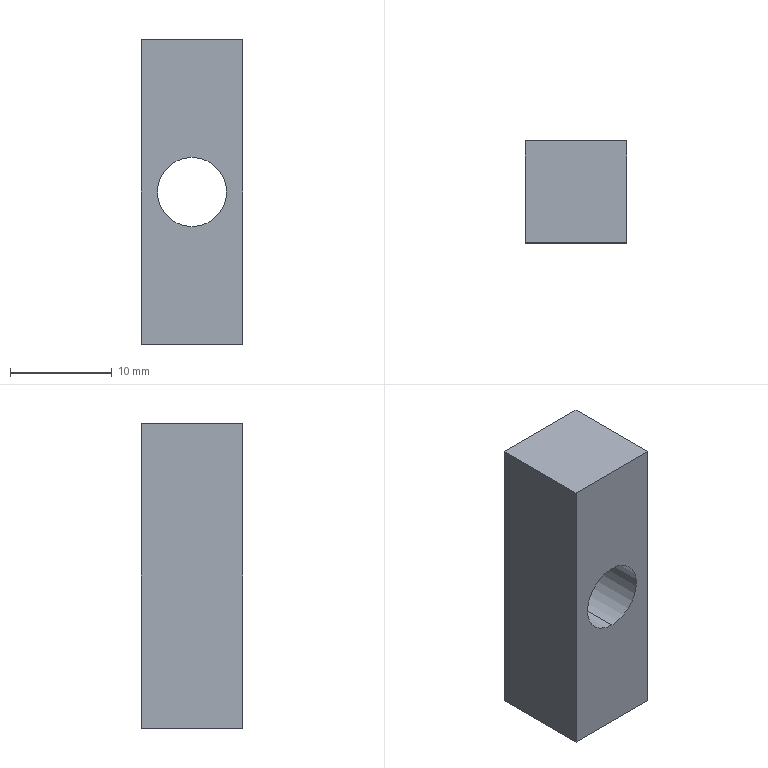Part | STEP file | 1 solid | 8 faces | box 10 x 10 x 30 mm | volume 2637 mm3 | plane 6 | cylinder 2 | commonest cylinder face diameters 6.8 x2
STEP:
#1=CARTESIAN_POINT('',(0.,0.,0.));
#2=DIRECTION('',(0.,0.,1.));
#3=DIRECTION('',(1.,0.,0.));
#4=AXIS2_PLACEMENT_3D('',#1,#2,#3);
#5=CARTESIAN_POINT('',(0.,10.,3.4));
#6=VERTEX_POINT('',#5);
#7=CARTESIAN_POINT('',(0.,10.,-3.4));
#8=VERTEX_POINT('',#7);
#9=CARTESIAN_POINT('',(0.,10.,0.));
#10=DIRECTION('',(0.,1.,0.));
#11=DIRECTION('',(0.,0.,1.));
#12=AXIS2_PLACEMENT_3D('',#9,#10,#11);
#13=CIRCLE('',#12,3.4);
#14=CARTESIAN_POINT('',(0.,10.,0.));
#15=DIRECTION('',(0.,1.,0.));
#16=DIRECTION('',(0.,0.,1.));
#17=AXIS2_PLACEMENT_3D('',#14,#15,#16);
#18=CYLINDRICAL_SURFACE('',#17,3.4);
#19=CARTESIAN_POINT('',(0.,0.));
#20=DIRECTION('',(1.,0.));
#21=VECTOR('',#20,1.);
#22=LINE('',#19,#21);
#23=(GEOMETRIC_REPRESENTATION_CONTEXT(2)PARAMETRIC_REPRESENTATION_CONTEXT()REPRESENTATION_CONTEXT('',''));
#24=DEFINITIONAL_REPRESENTATION('',(#22),#23);
#25=PCURVE('',#18,#24);
#26=CARTESIAN_POINT('',(0.,10.,0.));
#27=DIRECTION('',(0.,-1.,0.));
#28=DIRECTION('',(0.,0.,-1.));
#29=AXIS2_PLACEMENT_3D('',#26,#27,#28);
#30=PLANE('',#29);
#31=CARTESIAN_POINT('',(-3.4,0.));
#32=CARTESIAN_POINT('',(-3.4,5.889));
#33=CARTESIAN_POINT('',(1.7,2.944));
#34=CARTESIAN_POINT('',(6.8,0.));
#35=CARTESIAN_POINT('',(1.7,-2.944));
#36=CARTESIAN_POINT('',(-3.4,-5.889));
#37=CARTESIAN_POINT('',(-3.4,0.));
#38=(BOUNDED_CURVE()B_SPLINE_CURVE(2,(#31,#32,#33,#34,#35,#36,#37),.UNSPECIFIED.,.T.,.F.)B_SPLINE_CURVE_WITH_KNOTS((1,2,2,2,2,1),(-2.094,0.,2.094,4.189,6.283,8.378),.UNSPECIFIED.)CURVE()GEOMETRIC_REPRESENTATION_ITEM()RATIONAL_B_SPLINE_CURVE((1.,0.5,1.,0.5,1.,0.5,1.))REPRESENTATION_ITEM(''));
#39=(GEOMETRIC_REPRESENTATION_CONTEXT(2)PARAMETRIC_REPRESENTATION_CONTEXT()REPRESENTATION_CONTEXT('',''));
#40=DEFINITIONAL_REPRESENTATION('',(#38),#39);
#41=PCURVE('',#30,#40);
#42=SURFACE_CURVE('',#13,(#25,#41),.PCURVE_S1.);
#43=EDGE_CURVE('',#6,#8,#42,.T.);
#44=ORIENTED_EDGE('',*,*,#43,.F.);
#45=CARTESIAN_POINT('',(0.,0.,3.4));
#46=VERTEX_POINT('',#45);
#47=CARTESIAN_POINT('',(0.,10.,3.4));
#48=DIRECTION('',(0.,1.,0.));
#49=VECTOR('',#48,1.);
#50=LINE('',#47,#49);
#51=CARTESIAN_POINT('',(0.,0.));
#52=DIRECTION('',(0.,1.));
#53=VECTOR('',#52,1.);
#54=LINE('',#51,#53);
#55=(GEOMETRIC_REPRESENTATION_CONTEXT(2)PARAMETRIC_REPRESENTATION_CONTEXT()REPRESENTATION_CONTEXT('',''));
#56=DEFINITIONAL_REPRESENTATION('',(#54),#55);
#57=PCURVE('',#18,#56);
#58=CARTESIAN_POINT('',(0.,10.,0.));
#59=DIRECTION('',(0.,1.,0.));
#60=DIRECTION('',(0.,0.,1.));
#61=AXIS2_PLACEMENT_3D('',#58,#59,#60);
#62=CYLINDRICAL_SURFACE('',#61,3.4);
#63=CARTESIAN_POINT('',(6.283,0.));
#64=DIRECTION('',(0.,1.));
#65=VECTOR('',#64,1.);
#66=LINE('',#63,#65);
#67=(GEOMETRIC_REPRESENTATION_CONTEXT(2)PARAMETRIC_REPRESENTATION_CONTEXT()REPRESENTATION_CONTEXT('',''));
#68=DEFINITIONAL_REPRESENTATION('',(#66),#67);
#69=PCURVE('',#62,#68);
#70=SURFACE_CURVE('',#50,(#57,#69),.PCURVE_S1.);
#71=EDGE_CURVE('',#46,#6,#70,.T.);
#72=ORIENTED_EDGE('',*,*,#71,.F.);
#73=CARTESIAN_POINT('',(0.,0.,-3.4));
#74=VERTEX_POINT('',#73);
#75=CARTESIAN_POINT('',(0.,0.,0.));
#76=DIRECTION('',(0.,-1.,0.));
#77=DIRECTION('',(0.,0.,-1.));
#78=AXIS2_PLACEMENT_3D('',#75,#76,#77);
#79=CIRCLE('',#78,3.4);
#80=CARTESIAN_POINT('',(3.142,-10.));
#81=DIRECTION('',(-1.,0.));
#82=VECTOR('',#81,1.);
#83=LINE('',#80,#82);
#84=(GEOMETRIC_REPRESENTATION_CONTEXT(2)PARAMETRIC_REPRESENTATION_CONTEXT()REPRESENTATION_CONTEXT('',''));
#85=DEFINITIONAL_REPRESENTATION('',(#83),#84);
#86=PCURVE('',#18,#85);
#87=CARTESIAN_POINT('',(0.,0.,0.));
#88=DIRECTION('',(0.,-1.,0.));
#89=DIRECTION('',(0.,0.,-1.));
#90=AXIS2_PLACEMENT_3D('',#87,#88,#89);
#91=PLANE('',#90);
#92=CARTESIAN_POINT('',(0.,0.));
#93=DIRECTION('',(1.,0.));
#94=AXIS2_PLACEMENT_2D('',#92,#93);
#95=CIRCLE('',#94,3.4);
#96=(GEOMETRIC_REPRESENTATION_CONTEXT(2)PARAMETRIC_REPRESENTATION_CONTEXT()REPRESENTATION_CONTEXT('',''));
#97=DEFINITIONAL_REPRESENTATION('',(#95),#96);
#98=PCURVE('',#91,#97);
#99=SURFACE_CURVE('',#79,(#86,#98),.PCURVE_S1.);
#100=EDGE_CURVE('',#74,#46,#99,.T.);
#101=ORIENTED_EDGE('',*,*,#100,.F.);
#102=CARTESIAN_POINT('',(0.,10.,-3.4));
#103=DIRECTION('',(0.,1.,0.));
#104=VECTOR('',#103,1.);
#105=LINE('',#102,#104);
#106=CARTESIAN_POINT('',(3.142,0.));
#107=DIRECTION('',(0.,1.));
#108=VECTOR('',#107,1.);
#109=LINE('',#106,#108);
#110=(GEOMETRIC_REPRESENTATION_CONTEXT(2)PARAMETRIC_REPRESENTATION_CONTEXT()REPRESENTATION_CONTEXT('',''));
#111=DEFINITIONAL_REPRESENTATION('',(#109),#110);
#112=PCURVE('',#18,#111);
#113=CARTESIAN_POINT('',(3.142,0.));
#114=DIRECTION('',(0.,1.));
#115=VECTOR('',#114,1.);
#116=LINE('',#113,#115);
#117=(GEOMETRIC_REPRESENTATION_CONTEXT(2)PARAMETRIC_REPRESENTATION_CONTEXT()REPRESENTATION_CONTEXT('',''));
#118=DEFINITIONAL_REPRESENTATION('',(#116),#117);
#119=PCURVE('',#62,#118);
#120=SURFACE_CURVE('',#105,(#112,#119),.PCURVE_S1.);
#121=EDGE_CURVE('',#74,#8,#120,.T.);
#122=ORIENTED_EDGE('',*,*,#121,.T.);
#123=EDGE_LOOP('',(#44,#72,#101,#122));
#124=FACE_BOUND('',#123,.F.);
#125=ADVANCED_FACE('',(#124),#18,.F.);
#126=CARTESIAN_POINT('',(0.,0.,0.));
#127=DIRECTION('',(0.,-1.,0.));
#128=DIRECTION('',(0.,0.,-1.));
#129=AXIS2_PLACEMENT_3D('',#126,#127,#128);
#130=CIRCLE('',#129,3.4);
#131=CARTESIAN_POINT('',(0.,0.));
#132=DIRECTION('',(1.,0.));
#133=AXIS2_PLACEMENT_2D('',#131,#132);
#134=CIRCLE('',#133,3.4);
#135=(GEOMETRIC_REPRESENTATION_CONTEXT(2)PARAMETRIC_REPRESENTATION_CONTEXT()REPRESENTATION_CONTEXT('',''));
#136=DEFINITIONAL_REPRESENTATION('',(#134),#135);
#137=PCURVE('',#91,#136);
#138=CARTESIAN_POINT('',(9.425,-10.));
#139=DIRECTION('',(-1.,0.));
#140=VECTOR('',#139,1.);
#141=LINE('',#138,#140);
#142=(GEOMETRIC_REPRESENTATION_CONTEXT(2)PARAMETRIC_REPRESENTATION_CONTEXT()REPRESENTATION_CONTEXT('',''));
#143=DEFINITIONAL_REPRESENTATION('',(#141),#142);
#144=PCURVE('',#62,#143);
#145=SURFACE_CURVE('',#130,(#137,#144),.PCURVE_S1.);
#146=EDGE_CURVE('',#46,#74,#145,.T.);
#147=ORIENTED_EDGE('',*,*,#146,.F.);
#148=ORIENTED_EDGE('',*,*,#100,.F.);
#149=EDGE_LOOP('',(#147,#148));
#150=FACE_BOUND('',#149,.T.);
#151=CARTESIAN_POINT('',(5.,0.,15.));
#152=VERTEX_POINT('',#151);
#153=CARTESIAN_POINT('',(5.,0.,-15.));
#154=VERTEX_POINT('',#153);
#155=CARTESIAN_POINT('',(5.,0.,15.));
#156=DIRECTION('',(0.,0.,-1.));
#157=VECTOR('',#156,1.);
#158=LINE('',#155,#157);
#159=CARTESIAN_POINT('',(-15.,5.));
#160=DIRECTION('',(1.,0.));
#161=VECTOR('',#160,1.);
#162=LINE('',#159,#161);
#163=(GEOMETRIC_REPRESENTATION_CONTEXT(2)PARAMETRIC_REPRESENTATION_CONTEXT()REPRESENTATION_CONTEXT('',''));
#164=DEFINITIONAL_REPRESENTATION('',(#162),#163);
#165=PCURVE('',#91,#164);
#166=CARTESIAN_POINT('',(5.,10.,15.));
#167=DIRECTION('',(-1.,0.,0.));
#168=DIRECTION('',(0.,0.,1.));
#169=AXIS2_PLACEMENT_3D('',#166,#167,#168);
#170=PLANE('',#169);
#171=CARTESIAN_POINT('',(0.,-10.));
#172=DIRECTION('',(-1.,0.));
#173=VECTOR('',#172,1.);
#174=LINE('',#171,#173);
#175=(GEOMETRIC_REPRESENTATION_CONTEXT(2)PARAMETRIC_REPRESENTATION_CONTEXT()REPRESENTATION_CONTEXT('',''));
#176=DEFINITIONAL_REPRESENTATION('',(#174),#175);
#177=PCURVE('',#170,#176);
#178=SURFACE_CURVE('',#158,(#165,#177),.PCURVE_S1.);
#179=EDGE_CURVE('',#152,#154,#178,.T.);
#180=ORIENTED_EDGE('',*,*,#179,.F.);
#181=CARTESIAN_POINT('',(-5.,0.,15.));
#182=VERTEX_POINT('',#181);
#183=CARTESIAN_POINT('',(-5.,0.,15.));
#184=DIRECTION('',(1.,0.,0.));
#185=VECTOR('',#184,1.);
#186=LINE('',#183,#185);
#187=CARTESIAN_POINT('',(-15.,-5.));
#188=DIRECTION('',(0.,1.));
#189=VECTOR('',#188,1.);
#190=LINE('',#187,#189);
#191=(GEOMETRIC_REPRESENTATION_CONTEXT(2)PARAMETRIC_REPRESENTATION_CONTEXT()REPRESENTATION_CONTEXT('',''));
#192=DEFINITIONAL_REPRESENTATION('',(#190),#191);
#193=PCURVE('',#91,#192);
#194=CARTESIAN_POINT('',(-5.,10.,15.));
#195=DIRECTION('',(0.,0.,-1.));
#196=DIRECTION('',(0.,-1.,0.));
#197=AXIS2_PLACEMENT_3D('',#194,#195,#196);
#198=PLANE('',#197);
#199=CARTESIAN_POINT('',(10.,0.));
#200=DIRECTION('',(0.,-1.));
#201=VECTOR('',#200,1.);
#202=LINE('',#199,#201);
#203=(GEOMETRIC_REPRESENTATION_CONTEXT(2)PARAMETRIC_REPRESENTATION_CONTEXT()REPRESENTATION_CONTEXT('',''));
#204=DEFINITIONAL_REPRESENTATION('',(#202),#203);
#205=PCURVE('',#198,#204);
#206=SURFACE_CURVE('',#186,(#193,#205),.PCURVE_S1.);
#207=EDGE_CURVE('',#182,#152,#206,.T.);
#208=ORIENTED_EDGE('',*,*,#207,.F.);
#209=CARTESIAN_POINT('',(-5.,0.,-15.));
#210=VERTEX_POINT('',#209);
#211=CARTESIAN_POINT('',(-5.,0.,15.));
#212=DIRECTION('',(0.,0.,1.));
#213=VECTOR('',#212,1.);
#214=LINE('',#211,#213);
#215=CARTESIAN_POINT('',(-15.,-5.));
#216=DIRECTION('',(-1.,0.));
#217=VECTOR('',#216,1.);
#218=LINE('',#215,#217);
#219=(GEOMETRIC_REPRESENTATION_CONTEXT(2)PARAMETRIC_REPRESENTATION_CONTEXT()REPRESENTATION_CONTEXT('',''));
#220=DEFINITIONAL_REPRESENTATION('',(#218),#219);
#221=PCURVE('',#91,#220);
#222=CARTESIAN_POINT('',(-5.,10.,15.));
#223=DIRECTION('',(1.,0.,0.));
#224=DIRECTION('',(0.,1.,0.));
#225=AXIS2_PLACEMENT_3D('',#222,#223,#224);
#226=PLANE('',#225);
#227=CARTESIAN_POINT('',(-10.,0.));
#228=DIRECTION('',(0.,1.));
#229=VECTOR('',#228,1.);
#230=LINE('',#227,#229);
#231=(GEOMETRIC_REPRESENTATION_CONTEXT(2)PARAMETRIC_REPRESENTATION_CONTEXT()REPRESENTATION_CONTEXT('',''));
#232=DEFINITIONAL_REPRESENTATION('',(#230),#231);
#233=PCURVE('',#226,#232);
#234=SURFACE_CURVE('',#214,(#221,#233),.PCURVE_S1.);
#235=EDGE_CURVE('',#210,#182,#234,.T.);
#236=ORIENTED_EDGE('',*,*,#235,.F.);
#237=CARTESIAN_POINT('',(-5.,0.,-15.));
#238=DIRECTION('',(-1.,0.,0.));
#239=VECTOR('',#238,1.);
#240=LINE('',#237,#239);
#241=CARTESIAN_POINT('',(15.,-5.));
#242=DIRECTION('',(0.,-1.));
#243=VECTOR('',#242,1.);
#244=LINE('',#241,#243);
#245=(GEOMETRIC_REPRESENTATION_CONTEXT(2)PARAMETRIC_REPRESENTATION_CONTEXT()REPRESENTATION_CONTEXT('',''));
#246=DEFINITIONAL_REPRESENTATION('',(#244),#245);
#247=PCURVE('',#91,#246);
#248=CARTESIAN_POINT('',(-5.,10.,-15.));
#249=DIRECTION('',(0.,0.,1.));
#250=DIRECTION('',(1.,0.,0.));
#251=AXIS2_PLACEMENT_3D('',#248,#249,#250);
#252=PLANE('',#251);
#253=CARTESIAN_POINT('',(0.,-10.));
#254=DIRECTION('',(-1.,0.));
#255=VECTOR('',#254,1.);
#256=LINE('',#253,#255);
#257=(GEOMETRIC_REPRESENTATION_CONTEXT(2)PARAMETRIC_REPRESENTATION_CONTEXT()REPRESENTATION_CONTEXT('',''));
#258=DEFINITIONAL_REPRESENTATION('',(#256),#257);
#259=PCURVE('',#252,#258);
#260=SURFACE_CURVE('',#240,(#247,#259),.PCURVE_S1.);
#261=EDGE_CURVE('',#154,#210,#260,.T.);
#262=ORIENTED_EDGE('',*,*,#261,.F.);
#263=EDGE_LOOP('',(#180,#208,#236,#262));
#264=FACE_BOUND('',#263,.T.);
#265=ADVANCED_FACE('',(#150,#264),#91,.T.);
#266=ORIENTED_EDGE('',*,*,#43,.F.);
#267=CARTESIAN_POINT('',(0.,10.,0.));
#268=DIRECTION('',(0.,1.,0.));
#269=DIRECTION('',(0.,0.,1.));
#270=AXIS2_PLACEMENT_3D('',#267,#268,#269);
#271=CIRCLE('',#270,3.4);
#272=CARTESIAN_POINT('',(-3.4,0.));
#273=CARTESIAN_POINT('',(-3.4,5.889));
#274=CARTESIAN_POINT('',(1.7,2.944));
#275=CARTESIAN_POINT('',(6.8,0.));
#276=CARTESIAN_POINT('',(1.7,-2.944));
#277=CARTESIAN_POINT('',(-3.4,-5.889));
#278=CARTESIAN_POINT('',(-3.4,0.));
#279=(BOUNDED_CURVE()B_SPLINE_CURVE(2,(#272,#273,#274,#275,#276,#277,#278),.UNSPECIFIED.,.T.,.F.)B_SPLINE_CURVE_WITH_KNOTS((1,2,2,2,2,1),(-2.094,0.,2.094,4.189,6.283,8.378),.UNSPECIFIED.)CURVE()GEOMETRIC_REPRESENTATION_ITEM()RATIONAL_B_SPLINE_CURVE((1.,0.5,1.,0.5,1.,0.5,1.))REPRESENTATION_ITEM(''));
#280=(GEOMETRIC_REPRESENTATION_CONTEXT(2)PARAMETRIC_REPRESENTATION_CONTEXT()REPRESENTATION_CONTEXT('',''));
#281=DEFINITIONAL_REPRESENTATION('',(#279),#280);
#282=PCURVE('',#30,#281);
#283=CARTESIAN_POINT('',(0.,0.));
#284=DIRECTION('',(1.,0.));
#285=VECTOR('',#284,1.);
#286=LINE('',#283,#285);
#287=(GEOMETRIC_REPRESENTATION_CONTEXT(2)PARAMETRIC_REPRESENTATION_CONTEXT()REPRESENTATION_CONTEXT('',''));
#288=DEFINITIONAL_REPRESENTATION('',(#286),#287);
#289=PCURVE('',#62,#288);
#290=SURFACE_CURVE('',#271,(#282,#289),.PCURVE_S1.);
#291=EDGE_CURVE('',#8,#6,#290,.T.);
#292=ORIENTED_EDGE('',*,*,#291,.F.);
#293=EDGE_LOOP('',(#266,#292));
#294=FACE_BOUND('',#293,.T.);
#295=CARTESIAN_POINT('',(5.,10.,15.));
#296=VERTEX_POINT('',#295);
#297=CARTESIAN_POINT('',(5.,10.,-15.));
#298=VERTEX_POINT('',#297);
#299=CARTESIAN_POINT('',(5.,10.,15.));
#300=DIRECTION('',(0.,0.,-1.));
#301=VECTOR('',#300,1.);
#302=LINE('',#299,#301);
#303=CARTESIAN_POINT('',(-15.,5.));
#304=DIRECTION('',(1.,0.));
#305=VECTOR('',#304,1.);
#306=LINE('',#303,#305);
#307=(GEOMETRIC_REPRESENTATION_CONTEXT(2)PARAMETRIC_REPRESENTATION_CONTEXT()REPRESENTATION_CONTEXT('',''));
#308=DEFINITIONAL_REPRESENTATION('',(#306),#307);
#309=PCURVE('',#30,#308);
#310=CARTESIAN_POINT('',(0.,0.));
#311=DIRECTION('',(-1.,0.));
#312=VECTOR('',#311,1.);
#313=LINE('',#310,#312);
#314=(GEOMETRIC_REPRESENTATION_CONTEXT(2)PARAMETRIC_REPRESENTATION_CONTEXT()REPRESENTATION_CONTEXT('',''));
#315=DEFINITIONAL_REPRESENTATION('',(#313),#314);
#316=PCURVE('',#170,#315);
#317=SURFACE_CURVE('',#302,(#309,#316),.PCURVE_S1.);
#318=EDGE_CURVE('',#296,#298,#317,.T.);
#319=ORIENTED_EDGE('',*,*,#318,.T.);
#320=CARTESIAN_POINT('',(-5.,10.,-15.));
#321=VERTEX_POINT('',#320);
#322=CARTESIAN_POINT('',(-5.,10.,-15.));
#323=DIRECTION('',(-1.,0.,0.));
#324=VECTOR('',#323,1.);
#325=LINE('',#322,#324);
#326=CARTESIAN_POINT('',(15.,-5.));
#327=DIRECTION('',(0.,-1.));
#328=VECTOR('',#327,1.);
#329=LINE('',#326,#328);
#330=(GEOMETRIC_REPRESENTATION_CONTEXT(2)PARAMETRIC_REPRESENTATION_CONTEXT()REPRESENTATION_CONTEXT('',''));
#331=DEFINITIONAL_REPRESENTATION('',(#329),#330);
#332=PCURVE('',#30,#331);
#333=CARTESIAN_POINT('',(0.,0.));
#334=DIRECTION('',(-1.,0.));
#335=VECTOR('',#334,1.);
#336=LINE('',#333,#335);
#337=(GEOMETRIC_REPRESENTATION_CONTEXT(2)PARAMETRIC_REPRESENTATION_CONTEXT()REPRESENTATION_CONTEXT('',''));
#338=DEFINITIONAL_REPRESENTATION('',(#336),#337);
#339=PCURVE('',#252,#338);
#340=SURFACE_CURVE('',#325,(#332,#339),.PCURVE_S1.);
#341=EDGE_CURVE('',#298,#321,#340,.T.);
#342=ORIENTED_EDGE('',*,*,#341,.T.);
#343=CARTESIAN_POINT('',(-5.,10.,15.));
#344=VERTEX_POINT('',#343);
#345=CARTESIAN_POINT('',(-5.,10.,15.));
#346=DIRECTION('',(0.,0.,1.));
#347=VECTOR('',#346,1.);
#348=LINE('',#345,#347);
#349=CARTESIAN_POINT('',(-15.,-5.));
#350=DIRECTION('',(-1.,0.));
#351=VECTOR('',#350,1.);
#352=LINE('',#349,#351);
#353=(GEOMETRIC_REPRESENTATION_CONTEXT(2)PARAMETRIC_REPRESENTATION_CONTEXT()REPRESENTATION_CONTEXT('',''));
#354=DEFINITIONAL_REPRESENTATION('',(#352),#353);
#355=PCURVE('',#30,#354);
#356=CARTESIAN_POINT('',(0.,0.));
#357=DIRECTION('',(0.,1.));
#358=VECTOR('',#357,1.);
#359=LINE('',#356,#358);
#360=(GEOMETRIC_REPRESENTATION_CONTEXT(2)PARAMETRIC_REPRESENTATION_CONTEXT()REPRESENTATION_CONTEXT('',''));
#361=DEFINITIONAL_REPRESENTATION('',(#359),#360);
#362=PCURVE('',#226,#361);
#363=SURFACE_CURVE('',#348,(#355,#362),.PCURVE_S1.);
#364=EDGE_CURVE('',#321,#344,#363,.T.);
#365=ORIENTED_EDGE('',*,*,#364,.T.);
#366=CARTESIAN_POINT('',(-5.,10.,15.));
#367=DIRECTION('',(1.,0.,0.));
#368=VECTOR('',#367,1.);
#369=LINE('',#366,#368);
#370=CARTESIAN_POINT('',(-15.,-5.));
#371=DIRECTION('',(0.,1.));
#372=VECTOR('',#371,1.);
#373=LINE('',#370,#372);
#374=(GEOMETRIC_REPRESENTATION_CONTEXT(2)PARAMETRIC_REPRESENTATION_CONTEXT()REPRESENTATION_CONTEXT('',''));
#375=DEFINITIONAL_REPRESENTATION('',(#373),#374);
#376=PCURVE('',#30,#375);
#377=CARTESIAN_POINT('',(0.,0.));
#378=DIRECTION('',(0.,-1.));
#379=VECTOR('',#378,1.);
#380=LINE('',#377,#379);
#381=(GEOMETRIC_REPRESENTATION_CONTEXT(2)PARAMETRIC_REPRESENTATION_CONTEXT()REPRESENTATION_CONTEXT('',''));
#382=DEFINITIONAL_REPRESENTATION('',(#380),#381);
#383=PCURVE('',#198,#382);
#384=SURFACE_CURVE('',#369,(#376,#383),.PCURVE_S1.);
#385=EDGE_CURVE('',#344,#296,#384,.T.);
#386=ORIENTED_EDGE('',*,*,#385,.T.);
#387=EDGE_LOOP('',(#319,#342,#365,#386));
#388=FACE_BOUND('',#387,.T.);
#389=ADVANCED_FACE('',(#294,#388),#30,.F.);
#390=ORIENTED_EDGE('',*,*,#207,.T.);
#391=CARTESIAN_POINT('',(5.,10.,15.));
#392=DIRECTION('',(0.,-1.,0.));
#393=VECTOR('',#392,1.);
#394=LINE('',#391,#393);
#395=CARTESIAN_POINT('',(0.,-10.));
#396=DIRECTION('',(1.,0.));
#397=VECTOR('',#396,1.);
#398=LINE('',#395,#397);
#399=(GEOMETRIC_REPRESENTATION_CONTEXT(2)PARAMETRIC_REPRESENTATION_CONTEXT()REPRESENTATION_CONTEXT('',''));
#400=DEFINITIONAL_REPRESENTATION('',(#398),#399);
#401=PCURVE('',#198,#400);
#402=CARTESIAN_POINT('',(0.,0.));
#403=DIRECTION('',(0.,-1.));
#404=VECTOR('',#403,1.);
#405=LINE('',#402,#404);
#406=(GEOMETRIC_REPRESENTATION_CONTEXT(2)PARAMETRIC_REPRESENTATION_CONTEXT()REPRESENTATION_CONTEXT('',''));
#407=DEFINITIONAL_REPRESENTATION('',(#405),#406);
#408=PCURVE('',#170,#407);
#409=SURFACE_CURVE('',#394,(#401,#408),.PCURVE_S1.);
#410=EDGE_CURVE('',#296,#152,#409,.T.);
#411=ORIENTED_EDGE('',*,*,#410,.F.);
#412=ORIENTED_EDGE('',*,*,#385,.F.);
#413=CARTESIAN_POINT('',(-5.,10.,15.));
#414=DIRECTION('',(0.,-1.,0.));
#415=VECTOR('',#414,1.);
#416=LINE('',#413,#415);
#417=CARTESIAN_POINT('',(0.,0.));
#418=DIRECTION('',(1.,0.));
#419=VECTOR('',#418,1.);
#420=LINE('',#417,#419);
#421=(GEOMETRIC_REPRESENTATION_CONTEXT(2)PARAMETRIC_REPRESENTATION_CONTEXT()REPRESENTATION_CONTEXT('',''));
#422=DEFINITIONAL_REPRESENTATION('',(#420),#421);
#423=PCURVE('',#198,#422);
#424=CARTESIAN_POINT('',(0.,0.));
#425=DIRECTION('',(-1.,0.));
#426=VECTOR('',#425,1.);
#427=LINE('',#424,#426);
#428=(GEOMETRIC_REPRESENTATION_CONTEXT(2)PARAMETRIC_REPRESENTATION_CONTEXT()REPRESENTATION_CONTEXT('',''));
#429=DEFINITIONAL_REPRESENTATION('',(#427),#428);
#430=PCURVE('',#226,#429);
#431=SURFACE_CURVE('',#416,(#423,#430),.PCURVE_S1.);
#432=EDGE_CURVE('',#344,#182,#431,.T.);
#433=ORIENTED_EDGE('',*,*,#432,.T.);
#434=EDGE_LOOP('',(#390,#411,#412,#433));
#435=FACE_BOUND('',#434,.T.);
#436=ADVANCED_FACE('',(#435),#198,.F.);
#437=ORIENTED_EDGE('',*,*,#235,.T.);
#438=ORIENTED_EDGE('',*,*,#432,.F.);
#439=ORIENTED_EDGE('',*,*,#364,.F.);
#440=CARTESIAN_POINT('',(-5.,10.,-15.));
#441=DIRECTION('',(0.,-1.,0.));
#442=VECTOR('',#441,1.);
#443=LINE('',#440,#442);
#444=CARTESIAN_POINT('',(0.,-30.));
#445=DIRECTION('',(-1.,0.));
#446=VECTOR('',#445,1.);
#447=LINE('',#444,#446);
#448=(GEOMETRIC_REPRESENTATION_CONTEXT(2)PARAMETRIC_REPRESENTATION_CONTEXT()REPRESENTATION_CONTEXT('',''));
#449=DEFINITIONAL_REPRESENTATION('',(#447),#448);
#450=PCURVE('',#226,#449);
#451=CARTESIAN_POINT('',(0.,0.));
#452=DIRECTION('',(0.,-1.));
#453=VECTOR('',#452,1.);
#454=LINE('',#451,#453);
#455=(GEOMETRIC_REPRESENTATION_CONTEXT(2)PARAMETRIC_REPRESENTATION_CONTEXT()REPRESENTATION_CONTEXT('',''));
#456=DEFINITIONAL_REPRESENTATION('',(#454),#455);
#457=PCURVE('',#252,#456);
#458=SURFACE_CURVE('',#443,(#450,#457),.PCURVE_S1.);
#459=EDGE_CURVE('',#321,#210,#458,.T.);
#460=ORIENTED_EDGE('',*,*,#459,.T.);
#461=EDGE_LOOP('',(#437,#438,#439,#460));
#462=FACE_BOUND('',#461,.T.);
#463=ADVANCED_FACE('',(#462),#226,.F.);
#464=ORIENTED_EDGE('',*,*,#261,.T.);
#465=ORIENTED_EDGE('',*,*,#459,.F.);
#466=ORIENTED_EDGE('',*,*,#341,.F.);
#467=CARTESIAN_POINT('',(5.,10.,-15.));
#468=DIRECTION('',(0.,-1.,0.));
#469=VECTOR('',#468,1.);
#470=LINE('',#467,#469);
#471=CARTESIAN_POINT('',(10.,0.));
#472=DIRECTION('',(0.,-1.));
#473=VECTOR('',#472,1.);
#474=LINE('',#471,#473);
#475=(GEOMETRIC_REPRESENTATION_CONTEXT(2)PARAMETRIC_REPRESENTATION_CONTEXT()REPRESENTATION_CONTEXT('',''));
#476=DEFINITIONAL_REPRESENTATION('',(#474),#475);
#477=PCURVE('',#252,#476);
#478=CARTESIAN_POINT('',(-30.,0.));
#479=DIRECTION('',(0.,-1.));
#480=VECTOR('',#479,1.);
#481=LINE('',#478,#480);
#482=(GEOMETRIC_REPRESENTATION_CONTEXT(2)PARAMETRIC_REPRESENTATION_CONTEXT()REPRESENTATION_CONTEXT('',''));
#483=DEFINITIONAL_REPRESENTATION('',(#481),#482);
#484=PCURVE('',#170,#483);
#485=SURFACE_CURVE('',#470,(#477,#484),.PCURVE_S1.);
#486=EDGE_CURVE('',#298,#154,#485,.T.);
#487=ORIENTED_EDGE('',*,*,#486,.T.);
#488=EDGE_LOOP('',(#464,#465,#466,#487));
#489=FACE_BOUND('',#488,.T.);
#490=ADVANCED_FACE('',(#489),#252,.F.);
#491=ORIENTED_EDGE('',*,*,#179,.T.);
#492=ORIENTED_EDGE('',*,*,#486,.F.);
#493=ORIENTED_EDGE('',*,*,#318,.F.);
#494=ORIENTED_EDGE('',*,*,#410,.T.);
#495=EDGE_LOOP('',(#491,#492,#493,#494));
#496=FACE_BOUND('',#495,.T.);
#497=ADVANCED_FACE('',(#496),#170,.F.);
#498=ORIENTED_EDGE('',*,*,#71,.T.);
#499=ORIENTED_EDGE('',*,*,#291,.F.);
#500=ORIENTED_EDGE('',*,*,#121,.F.);
#501=ORIENTED_EDGE('',*,*,#146,.F.);
#502=EDGE_LOOP('',(#498,#499,#500,#501));
#503=FACE_BOUND('',#502,.F.);
#504=ADVANCED_FACE('',(#503),#62,.F.);
#505=CLOSED_SHELL('',(#125,#265,#389,#436,#463,#490,#497,#504));
#506=MANIFOLD_SOLID_BREP('',#505);
#507=(LENGTH_UNIT()NAMED_UNIT(*)SI_UNIT(.MILLI.,.METRE.));
#508=UNCERTAINTY_MEASURE_WITH_UNIT(LENGTH_MEASURE(0.0000001),#507,'','');
#509=(NAMED_UNIT(*)PLANE_ANGLE_UNIT()SI_UNIT($,.RADIAN.));
#510=(NAMED_UNIT(*)SI_UNIT($,.STERADIAN.)SOLID_ANGLE_UNIT());
#511=(GEOMETRIC_REPRESENTATION_CONTEXT(3)GLOBAL_UNCERTAINTY_ASSIGNED_CONTEXT((#508))GLOBAL_UNIT_ASSIGNED_CONTEXT((#507,#509,#510))REPRESENTATION_CONTEXT('',''));
#512=ADVANCED_BREP_SHAPE_REPRESENTATION('',(#4,#506),#511);